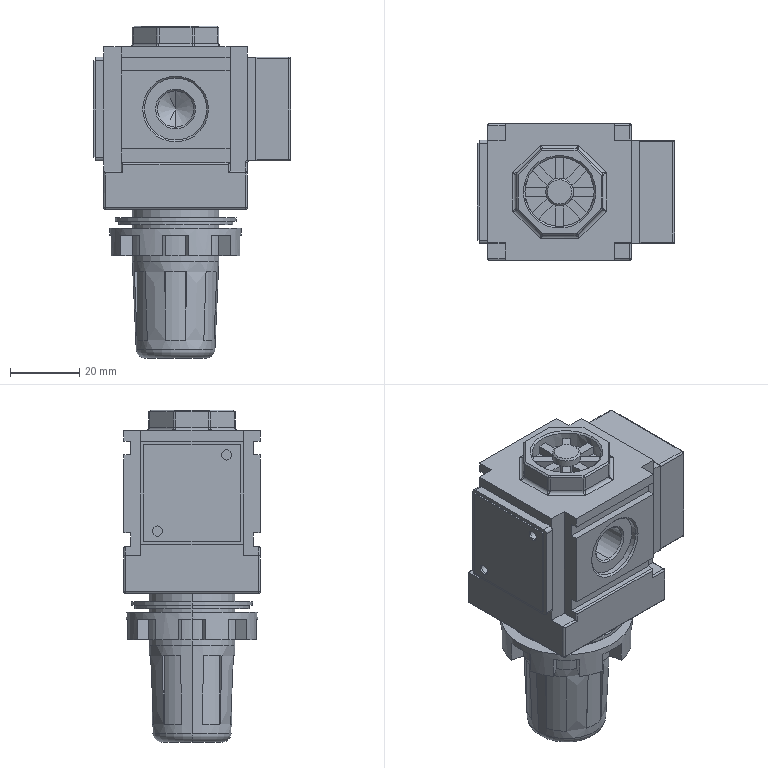Part | STEP file | Pressure regulating valve AR2000 | 4 solids | 363 faces | box 57 x 39.5 x 96 mm | volume 107387 mm3 | plane 208 | cylinder 107 | cone 26 | sphere 10 | spline 8 | torus 4 | commonest cylinder face diameters 1 x32 2 x20 3 x12 30 x9 23 x6 25 x6